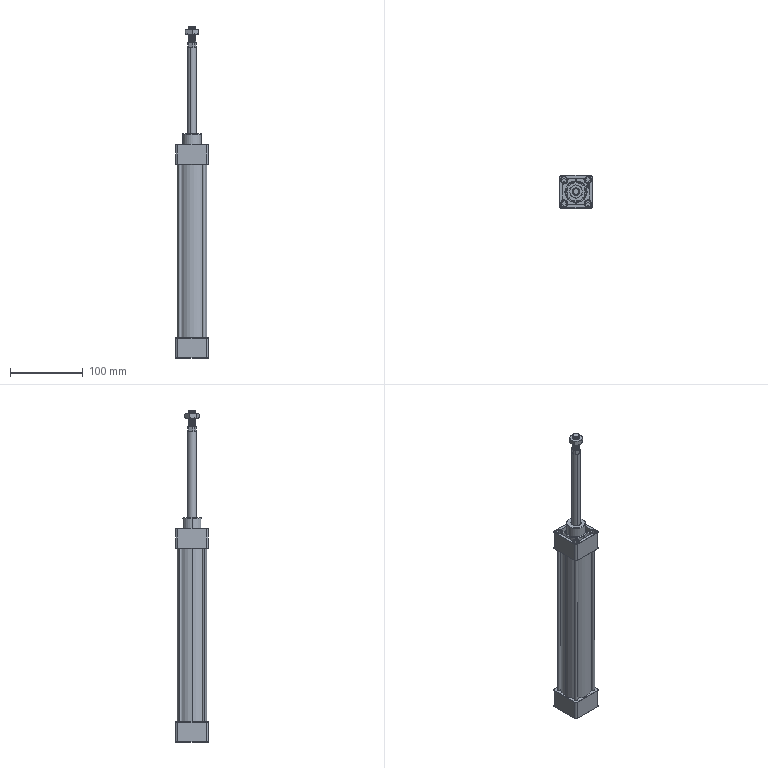Part | SolidWorks | 3 solids | 420 faces | box 45 x 45 x 455.652 mm | volume 288434 mm3 | plane 185 | cylinder 144 | cone 57 | torus 26 | spline 8 | commonest cylinder face diameters 9.147 x30 10 x26 8.6 x16 9 x16 2 x10 4.5 x8